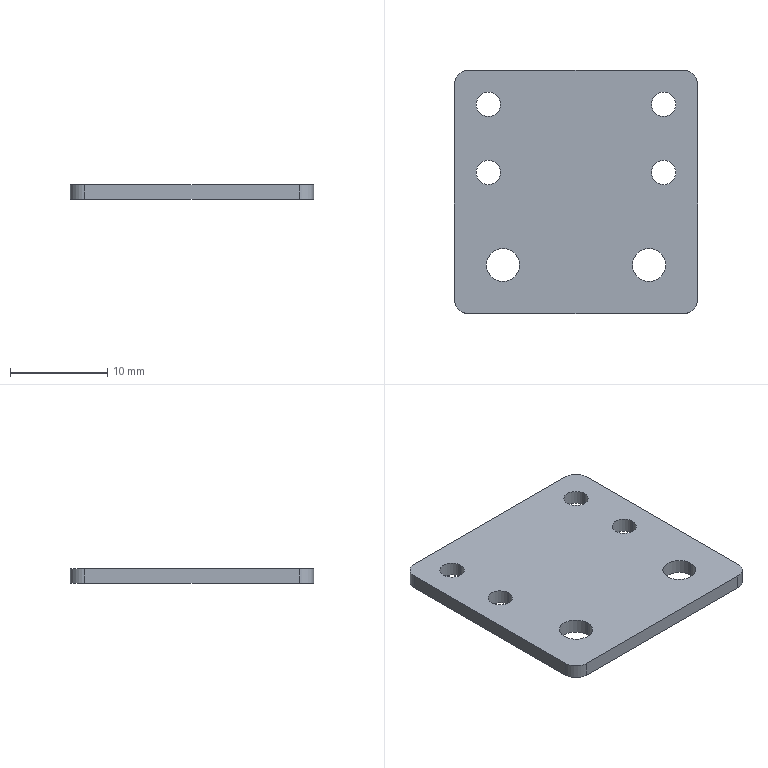Part | SolidWorks | features HoleWzd 2, Fillet 1, FlatPattern 1, SMBaseFlange 1, SheetMetal 1 | 1 solid | 22 faces | box 25 x 25 x 1.5 mm | volume 877.913 mm3 | cylinder 16 | plane 6 | commonest cylinder face diameters 2.5 x8 3 x4 3.4 x4
STEP:
#1=CARTESIAN_POINT('',(-9.2,-7.5,-1.5));
#2=VERTEX_POINT('',#1);
#3=CARTESIAN_POINT('',(-5.8,-7.5,-1.5));
#4=VERTEX_POINT('',#3);
#5=CARTESIAN_POINT('',(-7.5,-7.5,-1.5));
#6=DIRECTION('',(0.,0.,1.));
#7=DIRECTION('',(1.,0.,0.));
#8=AXIS2_PLACEMENT_3D('',#5,#6,#7);
#9=CIRCLE('',#8,1.7);
#10=EDGE_CURVE('',#2,#4,#9,.T.);
#11=ORIENTED_EDGE('',*,*,#10,.F.);
#12=CARTESIAN_POINT('',(-9.2,-7.5,0.));
#13=VERTEX_POINT('',#12);
#14=CARTESIAN_POINT('',(-9.2,-7.5,0.));
#15=DIRECTION('',(0.,0.,1.));
#16=VECTOR('',#15,1000.);
#17=LINE('',#14,#16);
#18=EDGE_CURVE('',#2,#13,#17,.T.);
#19=ORIENTED_EDGE('',*,*,#18,.T.);
#20=CARTESIAN_POINT('',(-5.8,-7.5,0.));
#21=VERTEX_POINT('',#20);
#22=CARTESIAN_POINT('',(-7.5,-7.5,0.));
#23=DIRECTION('',(0.,0.,1.));
#24=DIRECTION('',(1.,0.,0.));
#25=AXIS2_PLACEMENT_3D('',#22,#23,#24);
#26=CIRCLE('',#25,1.7);
#27=EDGE_CURVE('',#13,#21,#26,.T.);
#28=ORIENTED_EDGE('',*,*,#27,.T.);
#29=CARTESIAN_POINT('',(-5.8,-7.5,0.));
#30=DIRECTION('',(0.,0.,1.));
#31=VECTOR('',#30,1000.);
#32=LINE('',#29,#31);
#33=EDGE_CURVE('',#4,#21,#32,.T.);
#34=ORIENTED_EDGE('',*,*,#33,.F.);
#35=EDGE_LOOP('',(#11,#19,#28,#34));
#36=FACE_OUTER_BOUND('',#35,.T.);
#37=CARTESIAN_POINT('',(-7.5,-7.5,0.));
#38=DIRECTION('',(0.,0.,1.));
#39=DIRECTION('',(1.,0.,0.));
#40=AXIS2_PLACEMENT_3D('',#37,#38,#39);
#41=CYLINDRICAL_SURFACE('',#40,1.7);
#42=ADVANCED_FACE('',(#36),#41,.F.);
#43=CARTESIAN_POINT('',(5.8,-7.5,-1.5));
#44=VERTEX_POINT('',#43);
#45=CARTESIAN_POINT('',(9.2,-7.5,-1.5));
#46=VERTEX_POINT('',#45);
#47=CARTESIAN_POINT('',(7.5,-7.5,-1.5));
#48=DIRECTION('',(0.,0.,1.));
#49=DIRECTION('',(1.,0.,0.));
#50=AXIS2_PLACEMENT_3D('',#47,#48,#49);
#51=CIRCLE('',#50,1.7);
#52=EDGE_CURVE('',#44,#46,#51,.T.);
#53=ORIENTED_EDGE('',*,*,#52,.F.);
#54=CARTESIAN_POINT('',(5.8,-7.5,0.));
#55=VERTEX_POINT('',#54);
#56=CARTESIAN_POINT('',(5.8,-7.5,0.));
#57=DIRECTION('',(0.,0.,1.));
#58=VECTOR('',#57,1000.);
#59=LINE('',#56,#58);
#60=EDGE_CURVE('',#44,#55,#59,.T.);
#61=ORIENTED_EDGE('',*,*,#60,.T.);
#62=CARTESIAN_POINT('',(9.2,-7.5,0.));
#63=VERTEX_POINT('',#62);
#64=CARTESIAN_POINT('',(7.5,-7.5,0.));
#65=DIRECTION('',(0.,0.,1.));
#66=DIRECTION('',(1.,0.,0.));
#67=AXIS2_PLACEMENT_3D('',#64,#65,#66);
#68=CIRCLE('',#67,1.7);
#69=EDGE_CURVE('',#55,#63,#68,.T.);
#70=ORIENTED_EDGE('',*,*,#69,.T.);
#71=CARTESIAN_POINT('',(9.2,-7.5,0.));
#72=DIRECTION('',(0.,0.,1.));
#73=VECTOR('',#72,1000.);
#74=LINE('',#71,#73);
#75=EDGE_CURVE('',#46,#63,#74,.T.);
#76=ORIENTED_EDGE('',*,*,#75,.F.);
#77=EDGE_LOOP('',(#53,#61,#70,#76));
#78=FACE_OUTER_BOUND('',#77,.T.);
#79=CARTESIAN_POINT('',(7.5,-7.5,0.));
#80=DIRECTION('',(0.,0.,1.));
#81=DIRECTION('',(1.,0.,0.));
#82=AXIS2_PLACEMENT_3D('',#79,#80,#81);
#83=CYLINDRICAL_SURFACE('',#82,1.7);
#84=ADVANCED_FACE('',(#78),#83,.F.);
#85=CARTESIAN_POINT('',(-10.25,9.,-1.5));
#86=VERTEX_POINT('',#85);
#87=CARTESIAN_POINT('',(-7.75,9.,-1.5));
#88=VERTEX_POINT('',#87);
#89=CARTESIAN_POINT('',(-9.,9.,-1.5));
#90=DIRECTION('',(0.,0.,1.));
#91=DIRECTION('',(1.,0.,0.));
#92=AXIS2_PLACEMENT_3D('',#89,#90,#91);
#93=CIRCLE('',#92,1.25);
#94=EDGE_CURVE('',#86,#88,#93,.T.);
#95=ORIENTED_EDGE('',*,*,#94,.F.);
#96=CARTESIAN_POINT('',(-10.25,9.,0.));
#97=VERTEX_POINT('',#96);
#98=CARTESIAN_POINT('',(-10.25,9.,0.));
#99=DIRECTION('',(0.,0.,1.));
#100=VECTOR('',#99,1000.);
#101=LINE('',#98,#100);
#102=EDGE_CURVE('',#86,#97,#101,.T.);
#103=ORIENTED_EDGE('',*,*,#102,.T.);
#104=CARTESIAN_POINT('',(-7.75,9.,0.));
#105=VERTEX_POINT('',#104);
#106=CARTESIAN_POINT('',(-9.,9.,0.));
#107=DIRECTION('',(0.,0.,1.));
#108=DIRECTION('',(1.,0.,0.));
#109=AXIS2_PLACEMENT_3D('',#106,#107,#108);
#110=CIRCLE('',#109,1.25);
#111=EDGE_CURVE('',#97,#105,#110,.T.);
#112=ORIENTED_EDGE('',*,*,#111,.T.);
#113=CARTESIAN_POINT('',(-7.75,9.,0.));
#114=DIRECTION('',(0.,0.,1.));
#115=VECTOR('',#114,1000.);
#116=LINE('',#113,#115);
#117=EDGE_CURVE('',#88,#105,#116,.T.);
#118=ORIENTED_EDGE('',*,*,#117,.F.);
#119=EDGE_LOOP('',(#95,#103,#112,#118));
#120=FACE_OUTER_BOUND('',#119,.T.);
#121=CARTESIAN_POINT('',(-9.,9.,0.));
#122=DIRECTION('',(0.,0.,1.));
#123=DIRECTION('',(1.,0.,0.));
#124=AXIS2_PLACEMENT_3D('',#121,#122,#123);
#125=CYLINDRICAL_SURFACE('',#124,1.25);
#126=ADVANCED_FACE('',(#120),#125,.F.);
#127=CARTESIAN_POINT('',(-10.25,2.,-1.5));
#128=VERTEX_POINT('',#127);
#129=CARTESIAN_POINT('',(-7.75,2.,-1.5));
#130=VERTEX_POINT('',#129);
#131=CARTESIAN_POINT('',(-9.,2.,-1.5));
#132=DIRECTION('',(0.,0.,1.));
#133=DIRECTION('',(1.,0.,0.));
#134=AXIS2_PLACEMENT_3D('',#131,#132,#133);
#135=CIRCLE('',#134,1.25);
#136=EDGE_CURVE('',#128,#130,#135,.T.);
#137=ORIENTED_EDGE('',*,*,#136,.F.);
#138=CARTESIAN_POINT('',(-10.25,2.,0.));
#139=VERTEX_POINT('',#138);
#140=CARTESIAN_POINT('',(-10.25,2.,0.));
#141=DIRECTION('',(0.,0.,1.));
#142=VECTOR('',#141,1000.);
#143=LINE('',#140,#142);
#144=EDGE_CURVE('',#128,#139,#143,.T.);
#145=ORIENTED_EDGE('',*,*,#144,.T.);
#146=CARTESIAN_POINT('',(-7.75,2.,0.));
#147=VERTEX_POINT('',#146);
#148=CARTESIAN_POINT('',(-9.,2.,0.));
#149=DIRECTION('',(0.,0.,1.));
#150=DIRECTION('',(1.,0.,0.));
#151=AXIS2_PLACEMENT_3D('',#148,#149,#150);
#152=CIRCLE('',#151,1.25);
#153=EDGE_CURVE('',#139,#147,#152,.T.);
#154=ORIENTED_EDGE('',*,*,#153,.T.);
#155=CARTESIAN_POINT('',(-7.75,2.,0.));
#156=DIRECTION('',(0.,0.,1.));
#157=VECTOR('',#156,1000.);
#158=LINE('',#155,#157);
#159=EDGE_CURVE('',#130,#147,#158,.T.);
#160=ORIENTED_EDGE('',*,*,#159,.F.);
#161=EDGE_LOOP('',(#137,#145,#154,#160));
#162=FACE_OUTER_BOUND('',#161,.T.);
#163=CARTESIAN_POINT('',(-9.,2.,0.));
#164=DIRECTION('',(0.,0.,1.));
#165=DIRECTION('',(1.,0.,0.));
#166=AXIS2_PLACEMENT_3D('',#163,#164,#165);
#167=CYLINDRICAL_SURFACE('',#166,1.25);
#168=ADVANCED_FACE('',(#162),#167,.F.);
#169=CARTESIAN_POINT('',(7.75,2.,-1.5));
#170=VERTEX_POINT('',#169);
#171=CARTESIAN_POINT('',(10.25,2.,-1.5));
#172=VERTEX_POINT('',#171);
#173=CARTESIAN_POINT('',(9.,2.,-1.5));
#174=DIRECTION('',(0.,0.,1.));
#175=DIRECTION('',(1.,0.,0.));
#176=AXIS2_PLACEMENT_3D('',#173,#174,#175);
#177=CIRCLE('',#176,1.25);
#178=EDGE_CURVE('',#170,#172,#177,.T.);
#179=ORIENTED_EDGE('',*,*,#178,.F.);
#180=CARTESIAN_POINT('',(7.75,2.,0.));
#181=VERTEX_POINT('',#180);
#182=CARTESIAN_POINT('',(7.75,2.,0.));
#183=DIRECTION('',(0.,0.,1.));
#184=VECTOR('',#183,1000.);
#185=LINE('',#182,#184);
#186=EDGE_CURVE('',#170,#181,#185,.T.);
#187=ORIENTED_EDGE('',*,*,#186,.T.);
#188=CARTESIAN_POINT('',(10.25,2.,0.));
#189=VERTEX_POINT('',#188);
#190=CARTESIAN_POINT('',(9.,2.,0.));
#191=DIRECTION('',(0.,0.,1.));
#192=DIRECTION('',(1.,0.,0.));
#193=AXIS2_PLACEMENT_3D('',#190,#191,#192);
#194=CIRCLE('',#193,1.25);
#195=EDGE_CURVE('',#181,#189,#194,.T.);
#196=ORIENTED_EDGE('',*,*,#195,.T.);
#197=CARTESIAN_POINT('',(10.25,2.,0.));
#198=DIRECTION('',(0.,0.,1.));
#199=VECTOR('',#198,1000.);
#200=LINE('',#197,#199);
#201=EDGE_CURVE('',#172,#189,#200,.T.);
#202=ORIENTED_EDGE('',*,*,#201,.F.);
#203=EDGE_LOOP('',(#179,#187,#196,#202));
#204=FACE_OUTER_BOUND('',#203,.T.);
#205=CARTESIAN_POINT('',(9.,2.,0.));
#206=DIRECTION('',(0.,0.,1.));
#207=DIRECTION('',(1.,0.,0.));
#208=AXIS2_PLACEMENT_3D('',#205,#206,#207);
#209=CYLINDRICAL_SURFACE('',#208,1.25);
#210=ADVANCED_FACE('',(#204),#209,.F.);
#211=CARTESIAN_POINT('',(7.75,9.,-1.5));
#212=VERTEX_POINT('',#211);
#213=CARTESIAN_POINT('',(10.25,9.,-1.5));
#214=VERTEX_POINT('',#213);
#215=CARTESIAN_POINT('',(9.,9.,-1.5));
#216=DIRECTION('',(0.,0.,1.));
#217=DIRECTION('',(1.,0.,0.));
#218=AXIS2_PLACEMENT_3D('',#215,#216,#217);
#219=CIRCLE('',#218,1.25);
#220=EDGE_CURVE('',#212,#214,#219,.T.);
#221=ORIENTED_EDGE('',*,*,#220,.F.);
#222=CARTESIAN_POINT('',(7.75,9.,0.));
#223=VERTEX_POINT('',#222);
#224=CARTESIAN_POINT('',(7.75,9.,0.));
#225=DIRECTION('',(0.,0.,1.));
#226=VECTOR('',#225,1000.);
#227=LINE('',#224,#226);
#228=EDGE_CURVE('',#212,#223,#227,.T.);
#229=ORIENTED_EDGE('',*,*,#228,.T.);
#230=CARTESIAN_POINT('',(10.25,9.,0.));
#231=VERTEX_POINT('',#230);
#232=CARTESIAN_POINT('',(9.,9.,0.));
#233=DIRECTION('',(0.,0.,1.));
#234=DIRECTION('',(1.,0.,0.));
#235=AXIS2_PLACEMENT_3D('',#232,#233,#234);
#236=CIRCLE('',#235,1.25);
#237=EDGE_CURVE('',#223,#231,#236,.T.);
#238=ORIENTED_EDGE('',*,*,#237,.T.);
#239=CARTESIAN_POINT('',(10.25,9.,0.));
#240=DIRECTION('',(0.,0.,1.));
#241=VECTOR('',#240,1000.);
#242=LINE('',#239,#241);
#243=EDGE_CURVE('',#214,#231,#242,.T.);
#244=ORIENTED_EDGE('',*,*,#243,.F.);
#245=EDGE_LOOP('',(#221,#229,#238,#244));
#246=FACE_OUTER_BOUND('',#245,.T.);
#247=CARTESIAN_POINT('',(9.,9.,0.));
#248=DIRECTION('',(0.,0.,1.));
#249=DIRECTION('',(1.,0.,0.));
#250=AXIS2_PLACEMENT_3D('',#247,#248,#249);
#251=CYLINDRICAL_SURFACE('',#250,1.25);
#252=ADVANCED_FACE('',(#246),#251,.F.);
#253=CARTESIAN_POINT('',(12.5,-11.,0.));
#254=VERTEX_POINT('',#253);
#255=CARTESIAN_POINT('',(12.5,11.,0.));
#256=VERTEX_POINT('',#255);
#257=CARTESIAN_POINT('',(12.5,-12.5,0.));
#258=DIRECTION('',(0.,1.,0.));
#259=VECTOR('',#258,1000.);
#260=LINE('',#257,#259);
#261=EDGE_CURVE('',#254,#256,#260,.T.);
#262=ORIENTED_EDGE('',*,*,#261,.F.);
#263=CARTESIAN_POINT('',(12.5,-11.,-1.5));
#264=VERTEX_POINT('',#263);
#265=CARTESIAN_POINT('',(12.5,-11.,-1.5));
#266=DIRECTION('',(0.,0.,-1.));
#267=VECTOR('',#266,1000.);
#268=LINE('',#265,#267);
#269=EDGE_CURVE('',#254,#264,#268,.T.);
#270=ORIENTED_EDGE('',*,*,#269,.T.);
#271=CARTESIAN_POINT('',(12.5,11.,-1.5));
#272=VERTEX_POINT('',#271);
#273=CARTESIAN_POINT('',(12.5,-12.5,-1.5));
#274=DIRECTION('',(0.,1.,0.));
#275=VECTOR('',#274,1000.);
#276=LINE('',#273,#275);
#277=EDGE_CURVE('',#264,#272,#276,.T.);
#278=ORIENTED_EDGE('',*,*,#277,.T.);
#279=CARTESIAN_POINT('',(12.5,11.,-1.5));
#280=DIRECTION('',(0.,0.,1.));
#281=VECTOR('',#280,1000.);
#282=LINE('',#279,#281);
#283=EDGE_CURVE('',#272,#256,#282,.T.);
#284=ORIENTED_EDGE('',*,*,#283,.T.);
#285=EDGE_LOOP('',(#262,#270,#278,#284));
#286=FACE_OUTER_BOUND('',#285,.T.);
#287=CARTESIAN_POINT('',(12.5,-12.5,-1.5));
#288=DIRECTION('',(1.,0.,0.));
#289=DIRECTION('',(0.,0.,-1.));
#290=AXIS2_PLACEMENT_3D('',#287,#288,#289);
#291=PLANE('',#290);
#292=ADVANCED_FACE('',(#286),#291,.T.);
#293=CARTESIAN_POINT('',(-11.,-12.5,0.));
#294=VERTEX_POINT('',#293);
#295=CARTESIAN_POINT('',(11.,-12.5,0.));
#296=VERTEX_POINT('',#295);
#297=CARTESIAN_POINT('',(-12.5,-12.5,0.));
#298=DIRECTION('',(1.,0.,0.));
#299=VECTOR('',#298,1000.);
#300=LINE('',#297,#299);
#301=EDGE_CURVE('',#294,#296,#300,.T.);
#302=ORIENTED_EDGE('',*,*,#301,.F.);
#303=CARTESIAN_POINT('',(-11.,-12.5,-1.5));
#304=VERTEX_POINT('',#303);
#305=CARTESIAN_POINT('',(-11.,-12.5,-1.5));
#306=DIRECTION('',(0.,0.,-1.));
#307=VECTOR('',#306,1000.);
#308=LINE('',#305,#307);
#309=EDGE_CURVE('',#294,#304,#308,.T.);
#310=ORIENTED_EDGE('',*,*,#309,.T.);
#311=CARTESIAN_POINT('',(11.,-12.5,-1.5));
#312=VERTEX_POINT('',#311);
#313=CARTESIAN_POINT('',(-12.5,-12.5,-1.5));
#314=DIRECTION('',(1.,0.,0.));
#315=VECTOR('',#314,1000.);
#316=LINE('',#313,#315);
#317=EDGE_CURVE('',#304,#312,#316,.T.);
#318=ORIENTED_EDGE('',*,*,#317,.T.);
#319=CARTESIAN_POINT('',(11.,-12.5,-1.5));
#320=DIRECTION('',(0.,0.,1.));
#321=VECTOR('',#320,1000.);
#322=LINE('',#319,#321);
#323=EDGE_CURVE('',#312,#296,#322,.T.);
#324=ORIENTED_EDGE('',*,*,#323,.T.);
#325=EDGE_LOOP('',(#302,#310,#318,#324));
#326=FACE_OUTER_BOUND('',#325,.T.);
#327=CARTESIAN_POINT('',(-12.5,-12.5,-1.5));
#328=DIRECTION('',(0.,-1.,0.));
#329=DIRECTION('',(0.,0.,-1.));
#330=AXIS2_PLACEMENT_3D('',#327,#328,#329);
#331=PLANE('',#330);
#332=ADVANCED_FACE('',(#326),#331,.T.);
#333=CARTESIAN_POINT('',(-12.5,11.,-1.5));
#334=VERTEX_POINT('',#333);
#335=CARTESIAN_POINT('',(-12.5,-11.,-1.5));
#336=VERTEX_POINT('',#335);
#337=CARTESIAN_POINT('',(-12.5,-12.5,-1.5));
#338=DIRECTION('',(0.,-1.,0.));
#339=VECTOR('',#338,1000.);
#340=LINE('',#337,#339);
#341=EDGE_CURVE('',#334,#336,#340,.T.);
#342=ORIENTED_EDGE('',*,*,#341,.T.);
#343=CARTESIAN_POINT('',(-12.5,-11.,0.));
#344=VERTEX_POINT('',#343);
#345=CARTESIAN_POINT('',(-12.5,-11.,-1.5));
#346=DIRECTION('',(0.,0.,1.));
#347=VECTOR('',#346,1000.);
#348=LINE('',#345,#347);
#349=EDGE_CURVE('',#336,#344,#348,.T.);
#350=ORIENTED_EDGE('',*,*,#349,.T.);
#351=CARTESIAN_POINT('',(-12.5,11.,0.));
#352=VERTEX_POINT('',#351);
#353=CARTESIAN_POINT('',(-12.5,-12.5,0.));
#354=DIRECTION('',(0.,-1.,0.));
#355=VECTOR('',#354,1000.);
#356=LINE('',#353,#355);
#357=EDGE_CURVE('',#352,#344,#356,.T.);
#358=ORIENTED_EDGE('',*,*,#357,.F.);
#359=CARTESIAN_POINT('',(-12.5,11.,-1.5));
#360=DIRECTION('',(0.,0.,-1.));
#361=VECTOR('',#360,1000.);
#362=LINE('',#359,#361);
#363=EDGE_CURVE('',#352,#334,#362,.T.);
#364=ORIENTED_EDGE('',*,*,#363,.T.);
#365=EDGE_LOOP('',(#342,#350,#358,#364));
#366=FACE_OUTER_BOUND('',#365,.T.);
#367=CARTESIAN_POINT('',(-12.5,-12.5,-1.5));
#368=DIRECTION('',(-1.,0.,0.));
#369=DIRECTION('',(0.,0.,1.));
#370=AXIS2_PLACEMENT_3D('',#367,#368,#369);
#371=PLANE('',#370);
#372=ADVANCED_FACE('',(#366),#371,.T.);
#373=CARTESIAN_POINT('',(11.,12.5,-1.5));
#374=VERTEX_POINT('',#373);
#375=CARTESIAN_POINT('',(-11.,12.5,-1.5));
#376=VERTEX_POINT('',#375);
#377=CARTESIAN_POINT('',(-12.5,12.5,-1.5));
#378=DIRECTION('',(-1.,0.,0.));
#379=VECTOR('',#378,1000.);
#380=LINE('',#377,#379);
#381=EDGE_CURVE('',#374,#376,#380,.T.);
#382=ORIENTED_EDGE('',*,*,#381,.T.);
#383=CARTESIAN_POINT('',(-11.,12.5,0.));
#384=VERTEX_POINT('',#383);
#385=CARTESIAN_POINT('',(-11.,12.5,-1.5));
#386=DIRECTION('',(0.,0.,1.));
#387=VECTOR('',#386,1000.);
#388=LINE('',#385,#387);
#389=EDGE_CURVE('',#376,#384,#388,.T.);
#390=ORIENTED_EDGE('',*,*,#389,.T.);
#391=CARTESIAN_POINT('',(11.,12.5,0.));
#392=VERTEX_POINT('',#391);
#393=CARTESIAN_POINT('',(-12.5,12.5,0.));
#394=DIRECTION('',(-1.,0.,0.));
#395=VECTOR('',#394,1000.);
#396=LINE('',#393,#395);
#397=EDGE_CURVE('',#392,#384,#396,.T.);
#398=ORIENTED_EDGE('',*,*,#397,.F.);
#399=CARTESIAN_POINT('',(11.,12.5,-1.5));
#400=DIRECTION('',(0.,0.,-1.));
#401=VECTOR('',#400,1000.);
#402=LINE('',#399,#401);
#403=EDGE_CURVE('',#392,#374,#402,.T.);
#404=ORIENTED_EDGE('',*,*,#403,.T.);
#405=EDGE_LOOP('',(#382,#390,#398,#404));
#406=FACE_OUTER_BOUND('',#405,.T.);
#407=CARTESIAN_POINT('',(-12.5,12.5,-1.5));
#408=DIRECTION('',(0.,1.,0.));
#409=DIRECTION('',(0.,0.,1.));
#410=AXIS2_PLACEMENT_3D('',#407,#408,#409);
#411=PLANE('',#410);
#412=ADVANCED_FACE('',(#406),#411,.T.);
#413=CARTESIAN_POINT('',(-7.5,-7.5,-1.5));
#414=DIRECTION('',(0.,0.,1.));
#415=DIRECTION('',(1.,0.,0.));
#416=AXIS2_PLACEMENT_3D('',#413,#414,#415);
#417=CIRCLE('',#416,1.7);
#418=EDGE_CURVE('',#4,#2,#417,.T.);
#419=ORIENTED_EDGE('',*,*,#418,.T.);
#420=ORIENTED_EDGE('',*,*,#10,.T.);
#421=EDGE_LOOP('',(#419,#420));
#422=FACE_BOUND('',#421,.T.);
#423=CARTESIAN_POINT('',(7.5,-7.5,-1.5));
#424=DIRECTION('',(0.,0.,1.));
#425=DIRECTION('',(1.,0.,0.));
#426=AXIS2_PLACEMENT_3D('',#423,#424,#425);
#427=CIRCLE('',#426,1.7);
#428=EDGE_CURVE('',#46,#44,#427,.T.);
#429=ORIENTED_EDGE('',*,*,#428,.T.);
#430=ORIENTED_EDGE('',*,*,#52,.T.);
#431=EDGE_LOOP('',(#429,#430));
#432=FACE_BOUND('',#431,.T.);
#433=CARTESIAN_POINT('',(-9.,9.,-1.5));
#434=DIRECTION('',(0.,0.,1.));
#435=DIRECTION('',(1.,0.,0.));
#436=AXIS2_PLACEMENT_3D('',#433,#434,#435);
#437=CIRCLE('',#436,1.25);
#438=EDGE_CURVE('',#88,#86,#437,.T.);
#439=ORIENTED_EDGE('',*,*,#438,.T.);
#440=ORIENTED_EDGE('',*,*,#94,.T.);
#441=EDGE_LOOP('',(#439,#440));
#442=FACE_BOUND('',#441,.T.);
#443=CARTESIAN_POINT('',(-9.,2.,-1.5));
#444=DIRECTION('',(0.,0.,1.));
#445=DIRECTION('',(1.,0.,0.));
#446=AXIS2_PLACEMENT_3D('',#443,#444,#445);
#447=CIRCLE('',#446,1.25);
#448=EDGE_CURVE('',#130,#128,#447,.T.);
#449=ORIENTED_EDGE('',*,*,#448,.T.);
#450=ORIENTED_EDGE('',*,*,#136,.T.);
#451=EDGE_LOOP('',(#449,#450));
#452=FACE_BOUND('',#451,.T.);
#453=CARTESIAN_POINT('',(9.,2.,-1.5));
#454=DIRECTION('',(0.,0.,1.));
#455=DIRECTION('',(1.,0.,0.));
#456=AXIS2_PLACEMENT_3D('',#453,#454,#455);
#457=CIRCLE('',#456,1.25);
#458=EDGE_CURVE('',#172,#170,#457,.T.);
#459=ORIENTED_EDGE('',*,*,#458,.T.);
#460=ORIENTED_EDGE('',*,*,#178,.T.);
#461=EDGE_LOOP('',(#459,#460));
#462=FACE_BOUND('',#461,.T.);
#463=CARTESIAN_POINT('',(9.,9.,-1.5));
#464=DIRECTION('',(0.,0.,1.));
#465=DIRECTION('',(1.,0.,0.));
#466=AXIS2_PLACEMENT_3D('',#463,#464,#465);
#467=CIRCLE('',#466,1.25);
#468=EDGE_CURVE('',#214,#212,#467,.T.);
#469=ORIENTED_EDGE('',*,*,#468,.T.);
#470=ORIENTED_EDGE('',*,*,#220,.T.);
#471=EDGE_LOOP('',(#469,#470));
#472=FACE_BOUND('',#471,.T.);
#473=ORIENTED_EDGE('',*,*,#317,.F.);
#474=CARTESIAN_POINT('',(-11.,-11.,-1.5));
#475=DIRECTION('',(0.,0.,-1.));
#476=DIRECTION('',(-1.,0.,0.));
#477=AXIS2_PLACEMENT_3D('',#474,#475,#476);
#478=CIRCLE('',#477,1.5);
#479=EDGE_CURVE('',#304,#336,#478,.T.);
#480=ORIENTED_EDGE('',*,*,#479,.T.);
#481=ORIENTED_EDGE('',*,*,#341,.F.);
#482=CARTESIAN_POINT('',(-11.,11.,-1.5));
#483=DIRECTION('',(0.,0.,-1.));
#484=DIRECTION('',(-1.,0.,0.));
#485=AXIS2_PLACEMENT_3D('',#482,#483,#484);
#486=CIRCLE('',#485,1.5);
#487=EDGE_CURVE('',#334,#376,#486,.T.);
#488=ORIENTED_EDGE('',*,*,#487,.T.);
#489=ORIENTED_EDGE('',*,*,#381,.F.);
#490=CARTESIAN_POINT('',(11.,11.,-1.5));
#491=DIRECTION('',(0.,0.,-1.));
#492=DIRECTION('',(-1.,0.,0.));
#493=AXIS2_PLACEMENT_3D('',#490,#491,#492);
#494=CIRCLE('',#493,1.5);
#495=EDGE_CURVE('',#374,#272,#494,.T.);
#496=ORIENTED_EDGE('',*,*,#495,.T.);
#497=ORIENTED_EDGE('',*,*,#277,.F.);
#498=CARTESIAN_POINT('',(11.,-11.,-1.5));
#499=DIRECTION('',(0.,0.,-1.));
#500=DIRECTION('',(-1.,0.,0.));
#501=AXIS2_PLACEMENT_3D('',#498,#499,#500);
#502=CIRCLE('',#501,1.5);
#503=EDGE_CURVE('',#264,#312,#502,.T.);
#504=ORIENTED_EDGE('',*,*,#503,.T.);
#505=EDGE_LOOP('',(#473,#480,#481,#488,#489,#496,#497,#504));
#506=FACE_OUTER_BOUND('',#505,.T.);
#507=CARTESIAN_POINT('',(0.,0.,-1.5));
#508=DIRECTION('',(0.,0.,-1.));
#509=DIRECTION('',(-1.,0.,0.));
#510=AXIS2_PLACEMENT_3D('',#507,#508,#509);
#511=PLANE('',#510);
#512=ADVANCED_FACE('',(#422,#432,#442,#452,#462,#472,#506),#511,.T.);
#513=CARTESIAN_POINT('',(-7.5,-7.5,0.));
#514=DIRECTION('',(0.,0.,1.));
#515=DIRECTION('',(1.,0.,0.));
#516=AXIS2_PLACEMENT_3D('',#513,#514,#515);
#517=CIRCLE('',#516,1.7);
#518=EDGE_CURVE('',#21,#13,#517,.T.);
#519=ORIENTED_EDGE('',*,*,#518,.F.);
#520=ORIENTED_EDGE('',*,*,#27,.F.);
#521=EDGE_LOOP('',(#519,#520));
#522=FACE_BOUND('',#521,.T.);
#523=CARTESIAN_POINT('',(7.5,-7.5,0.));
#524=DIRECTION('',(0.,0.,1.));
#525=DIRECTION('',(1.,0.,0.));
#526=AXIS2_PLACEMENT_3D('',#523,#524,#525);
#527=CIRCLE('',#526,1.7);
#528=EDGE_CURVE('',#63,#55,#527,.T.);
#529=ORIENTED_EDGE('',*,*,#528,.F.);
#530=ORIENTED_EDGE('',*,*,#69,.F.);
#531=EDGE_LOOP('',(#529,#530));
#532=FACE_BOUND('',#531,.T.);
#533=CARTESIAN_POINT('',(-9.,9.,0.));
#534=DIRECTION('',(0.,0.,1.));
#535=DIRECTION('',(1.,0.,0.));
#536=AXIS2_PLACEMENT_3D('',#533,#534,#535);
#537=CIRCLE('',#536,1.25);
#538=EDGE_CURVE('',#105,#97,#537,.T.);
#539=ORIENTED_EDGE('',*,*,#538,.F.);
#540=ORIENTED_EDGE('',*,*,#111,.F.);
#541=EDGE_LOOP('',(#539,#540));
#542=FACE_BOUND('',#541,.T.);
#543=CARTESIAN_POINT('',(-9.,2.,0.));
#544=DIRECTION('',(0.,0.,1.));
#545=DIRECTION('',(1.,0.,0.));
#546=AXIS2_PLACEMENT_3D('',#543,#544,#545);
#547=CIRCLE('',#546,1.25);
#548=EDGE_CURVE('',#147,#139,#547,.T.);
#549=ORIENTED_EDGE('',*,*,#548,.F.);
#550=ORIENTED_EDGE('',*,*,#153,.F.);
#551=EDGE_LOOP('',(#549,#550));
#552=FACE_BOUND('',#551,.T.);
#553=CARTESIAN_POINT('',(9.,2.,0.));
#554=DIRECTION('',(0.,0.,1.));
#555=DIRECTION('',(1.,0.,0.));
#556=AXIS2_PLACEMENT_3D('',#553,#554,#555);
#557=CIRCLE('',#556,1.25);
#558=EDGE_CURVE('',#189,#181,#557,.T.);
#559=ORIENTED_EDGE('',*,*,#558,.F.);
#560=ORIENTED_EDGE('',*,*,#195,.F.);
#561=EDGE_LOOP('',(#559,#560));
#562=FACE_BOUND('',#561,.T.);
#563=CARTESIAN_POINT('',(9.,9.,0.));
#564=DIRECTION('',(0.,0.,1.));
#565=DIRECTION('',(1.,0.,0.));
#566=AXIS2_PLACEMENT_3D('',#563,#564,#565);
#567=CIRCLE('',#566,1.25);
#568=EDGE_CURVE('',#231,#223,#567,.T.);
#569=ORIENTED_EDGE('',*,*,#568,.F.);
#570=ORIENTED_EDGE('',*,*,#237,.F.);
#571=EDGE_LOOP('',(#569,#570));
#572=FACE_BOUND('',#571,.T.);
#573=ORIENTED_EDGE('',*,*,#357,.T.);
#574=CARTESIAN_POINT('',(-11.,-11.,0.));
#575=DIRECTION('',(0.,0.,1.));
#576=DIRECTION('',(-1.,0.,0.));
#577=AXIS2_PLACEMENT_3D('',#574,#575,#576);
#578=CIRCLE('',#577,1.5);
#579=EDGE_CURVE('',#344,#294,#578,.T.);
#580=ORIENTED_EDGE('',*,*,#579,.T.);
#581=ORIENTED_EDGE('',*,*,#301,.T.);
#582=CARTESIAN_POINT('',(11.,-11.,0.));
#583=DIRECTION('',(0.,0.,1.));
#584=DIRECTION('',(-1.,0.,0.));
#585=AXIS2_PLACEMENT_3D('',#582,#583,#584);
#586=CIRCLE('',#585,1.5);
#587=EDGE_CURVE('',#296,#254,#586,.T.);
#588=ORIENTED_EDGE('',*,*,#587,.T.);
#589=ORIENTED_EDGE('',*,*,#261,.T.);
#590=CARTESIAN_POINT('',(11.,11.,0.));
#591=DIRECTION('',(0.,0.,1.));
#592=DIRECTION('',(-1.,0.,0.));
#593=AXIS2_PLACEMENT_3D('',#590,#591,#592);
#594=CIRCLE('',#593,1.5);
#595=EDGE_CURVE('',#256,#392,#594,.T.);
#596=ORIENTED_EDGE('',*,*,#595,.T.);
#597=ORIENTED_EDGE('',*,*,#397,.T.);
#598=CARTESIAN_POINT('',(-11.,11.,0.));
#599=DIRECTION('',(0.,0.,1.));
#600=DIRECTION('',(-1.,0.,0.));
#601=AXIS2_PLACEMENT_3D('',#598,#599,#600);
#602=CIRCLE('',#601,1.5);
#603=EDGE_CURVE('',#384,#352,#602,.T.);
#604=ORIENTED_EDGE('',*,*,#603,.T.);
#605=EDGE_LOOP('',(#573,#580,#581,#588,#589,#596,#597,#604));
#606=FACE_OUTER_BOUND('',#605,.T.);
#607=CARTESIAN_POINT('',(0.,0.,0.));
#608=DIRECTION('',(0.,0.,-1.));
#609=DIRECTION('',(-1.,0.,0.));
#610=AXIS2_PLACEMENT_3D('',#607,#608,#609);
#611=PLANE('',#610);
#612=ADVANCED_FACE('',(#522,#532,#542,#552,#562,#572,#606),#611,.F.);
#613=ORIENTED_EDGE('',*,*,#479,.F.);
#614=ORIENTED_EDGE('',*,*,#309,.F.);
#615=ORIENTED_EDGE('',*,*,#579,.F.);
#616=ORIENTED_EDGE('',*,*,#349,.F.);
#617=EDGE_LOOP('',(#613,#614,#615,#616));
#618=FACE_OUTER_BOUND('',#617,.T.);
#619=CARTESIAN_POINT('',(-11.,-11.,-1.5));
#620=DIRECTION('',(0.,0.,1.));
#621=DIRECTION('',(1.,0.,0.));
#622=AXIS2_PLACEMENT_3D('',#619,#620,#621);
#623=CYLINDRICAL_SURFACE('',#622,1.5);
#624=ADVANCED_FACE('',(#618),#623,.T.);
#625=ORIENTED_EDGE('',*,*,#503,.F.);
#626=ORIENTED_EDGE('',*,*,#269,.F.);
#627=ORIENTED_EDGE('',*,*,#587,.F.);
#628=ORIENTED_EDGE('',*,*,#323,.F.);
#629=EDGE_LOOP('',(#625,#626,#627,#628));
#630=FACE_OUTER_BOUND('',#629,.T.);
#631=CARTESIAN_POINT('',(11.,-11.,-1.5));
#632=DIRECTION('',(0.,0.,1.));
#633=DIRECTION('',(1.,0.,0.));
#634=AXIS2_PLACEMENT_3D('',#631,#632,#633);
#635=CYLINDRICAL_SURFACE('',#634,1.5);
#636=ADVANCED_FACE('',(#630),#635,.T.);
#637=ORIENTED_EDGE('',*,*,#487,.F.);
#638=ORIENTED_EDGE('',*,*,#363,.F.);
#639=ORIENTED_EDGE('',*,*,#603,.F.);
#640=ORIENTED_EDGE('',*,*,#389,.F.);
#641=EDGE_LOOP('',(#637,#638,#639,#640));
#642=FACE_OUTER_BOUND('',#641,.T.);
#643=CARTESIAN_POINT('',(-11.,11.,-1.5));
#644=DIRECTION('',(0.,0.,1.));
#645=DIRECTION('',(1.,0.,0.));
#646=AXIS2_PLACEMENT_3D('',#643,#644,#645);
#647=CYLINDRICAL_SURFACE('',#646,1.5);
#648=ADVANCED_FACE('',(#642),#647,.T.);
#649=ORIENTED_EDGE('',*,*,#495,.F.);
#650=ORIENTED_EDGE('',*,*,#403,.F.);
#651=ORIENTED_EDGE('',*,*,#595,.F.);
#652=ORIENTED_EDGE('',*,*,#283,.F.);
#653=EDGE_LOOP('',(#649,#650,#651,#652));
#654=FACE_OUTER_BOUND('',#653,.T.);
#655=CARTESIAN_POINT('',(11.,11.,-1.5));
#656=DIRECTION('',(0.,0.,1.));
#657=DIRECTION('',(1.,0.,0.));
#658=AXIS2_PLACEMENT_3D('',#655,#656,#657);
#659=CYLINDRICAL_SURFACE('',#658,1.5);
#660=ADVANCED_FACE('',(#654),#659,.T.);
#661=ORIENTED_EDGE('',*,*,#228,.F.);
#662=ORIENTED_EDGE('',*,*,#468,.F.);
#663=ORIENTED_EDGE('',*,*,#243,.T.);
#664=ORIENTED_EDGE('',*,*,#568,.T.);
#665=EDGE_LOOP('',(#661,#662,#663,#664));
#666=FACE_OUTER_BOUND('',#665,.T.);
#667=CARTESIAN_POINT('',(9.,9.,0.));
#668=DIRECTION('',(0.,0.,1.));
#669=DIRECTION('',(1.,0.,0.));
#670=AXIS2_PLACEMENT_3D('',#667,#668,#669);
#671=CYLINDRICAL_SURFACE('',#670,1.25);
#672=ADVANCED_FACE('',(#666),#671,.F.);
#673=ORIENTED_EDGE('',*,*,#186,.F.);
#674=ORIENTED_EDGE('',*,*,#458,.F.);
#675=ORIENTED_EDGE('',*,*,#201,.T.);
#676=ORIENTED_EDGE('',*,*,#558,.T.);
#677=EDGE_LOOP('',(#673,#674,#675,#676));
#678=FACE_OUTER_BOUND('',#677,.T.);
#679=CARTESIAN_POINT('',(9.,2.,0.));
#680=DIRECTION('',(0.,0.,1.));
#681=DIRECTION('',(1.,0.,0.));
#682=AXIS2_PLACEMENT_3D('',#679,#680,#681);
#683=CYLINDRICAL_SURFACE('',#682,1.25);
#684=ADVANCED_FACE('',(#678),#683,.F.);
#685=ORIENTED_EDGE('',*,*,#144,.F.);
#686=ORIENTED_EDGE('',*,*,#448,.F.);
#687=ORIENTED_EDGE('',*,*,#159,.T.);
#688=ORIENTED_EDGE('',*,*,#548,.T.);
#689=EDGE_LOOP('',(#685,#686,#687,#688));
#690=FACE_OUTER_BOUND('',#689,.T.);
#691=CARTESIAN_POINT('',(-9.,2.,0.));
#692=DIRECTION('',(0.,0.,1.));
#693=DIRECTION('',(1.,0.,0.));
#694=AXIS2_PLACEMENT_3D('',#691,#692,#693);
#695=CYLINDRICAL_SURFACE('',#694,1.25);
#696=ADVANCED_FACE('',(#690),#695,.F.);
#697=ORIENTED_EDGE('',*,*,#102,.F.);
#698=ORIENTED_EDGE('',*,*,#438,.F.);
#699=ORIENTED_EDGE('',*,*,#117,.T.);
#700=ORIENTED_EDGE('',*,*,#538,.T.);
#701=EDGE_LOOP('',(#697,#698,#699,#700));
#702=FACE_OUTER_BOUND('',#701,.T.);
#703=CARTESIAN_POINT('',(-9.,9.,0.));
#704=DIRECTION('',(0.,0.,1.));
#705=DIRECTION('',(1.,0.,0.));
#706=AXIS2_PLACEMENT_3D('',#703,#704,#705);
#707=CYLINDRICAL_SURFACE('',#706,1.25);
#708=ADVANCED_FACE('',(#702),#707,.F.);
#709=ORIENTED_EDGE('',*,*,#60,.F.);
#710=ORIENTED_EDGE('',*,*,#428,.F.);
#711=ORIENTED_EDGE('',*,*,#75,.T.);
#712=ORIENTED_EDGE('',*,*,#528,.T.);
#713=EDGE_LOOP('',(#709,#710,#711,#712));
#714=FACE_OUTER_BOUND('',#713,.T.);
#715=CARTESIAN_POINT('',(7.5,-7.5,0.));
#716=DIRECTION('',(0.,0.,1.));
#717=DIRECTION('',(1.,0.,0.));
#718=AXIS2_PLACEMENT_3D('',#715,#716,#717);
#719=CYLINDRICAL_SURFACE('',#718,1.7);
#720=ADVANCED_FACE('',(#714),#719,.F.);
#721=ORIENTED_EDGE('',*,*,#18,.F.);
#722=ORIENTED_EDGE('',*,*,#418,.F.);
#723=ORIENTED_EDGE('',*,*,#33,.T.);
#724=ORIENTED_EDGE('',*,*,#518,.T.);
#725=EDGE_LOOP('',(#721,#722,#723,#724));
#726=FACE_OUTER_BOUND('',#725,.T.);
#727=CARTESIAN_POINT('',(-7.5,-7.5,0.));
#728=DIRECTION('',(0.,0.,1.));
#729=DIRECTION('',(1.,0.,0.));
#730=AXIS2_PLACEMENT_3D('',#727,#728,#729);
#731=CYLINDRICAL_SURFACE('',#730,1.7);
#732=ADVANCED_FACE('',(#726),#731,.F.);
#733=CLOSED_SHELL('',(#42,#84,#126,#168,#210,#252,#292,#332,#372,#412,#512,#612,#624,#636,#648,#660,#672,#684,#696,#708,#720,#732));
#734=MANIFOLD_SOLID_BREP('',#733);
#735=CARTESIAN_POINT('',(0.,0.,0.));
#736=DIRECTION('',(0.,0.,1.));
#737=DIRECTION('',(1.,0.,0.));
#738=AXIS2_PLACEMENT_3D('',#735,#736,#737);
#739=(LENGTH_UNIT()NAMED_UNIT(*)SI_UNIT(.MILLI.,.METRE.));
#740=UNCERTAINTY_MEASURE_WITH_UNIT(LENGTH_MEASURE(0.00001),#739,'','');
#741=(NAMED_UNIT(*)PLANE_ANGLE_UNIT()SI_UNIT($,.RADIAN.));
#742=(NAMED_UNIT(*)SI_UNIT($,.STERADIAN.)SOLID_ANGLE_UNIT());
#743=(GEOMETRIC_REPRESENTATION_CONTEXT(3)GLOBAL_UNCERTAINTY_ASSIGNED_CONTEXT((#740))GLOBAL_UNIT_ASSIGNED_CONTEXT((#739,#741,#742))REPRESENTATION_CONTEXT('',''));
#744=ADVANCED_BREP_SHAPE_REPRESENTATION('',(#734,#738),#743);